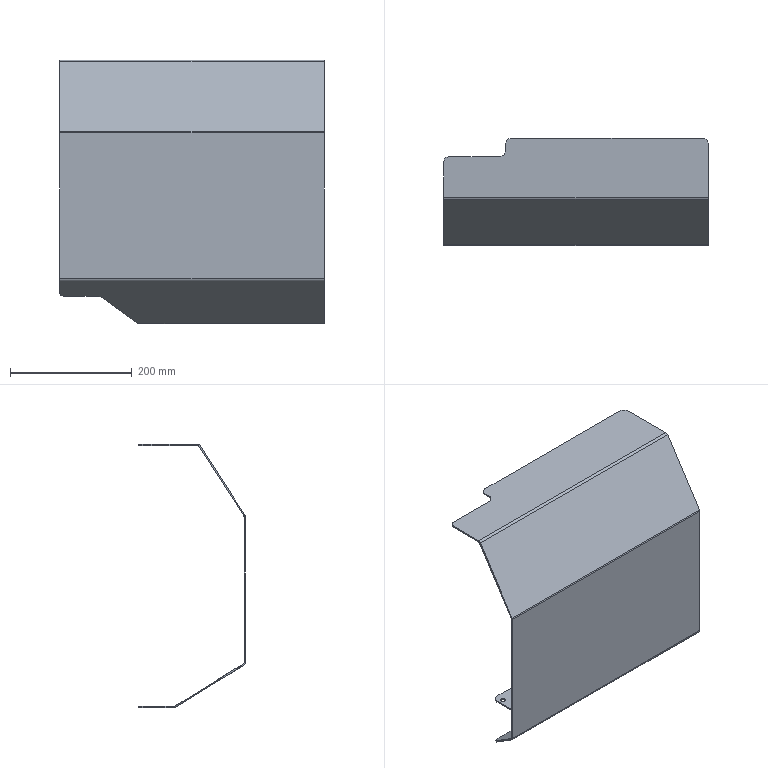Part | SolidWorks | features ICE 3, Fillet 1, FlatPattern 1, SMBaseFlange 1, SheetMetal 1 | 1 solid | 56 faces | box 436 x 176 x 434 mm | volume 633093 mm3 | plane 33 | cylinder 22 | spline 1 | commonest cylinder face diameters 20 x8 5 x4 9.6 x4 12.5 x4 8 x2